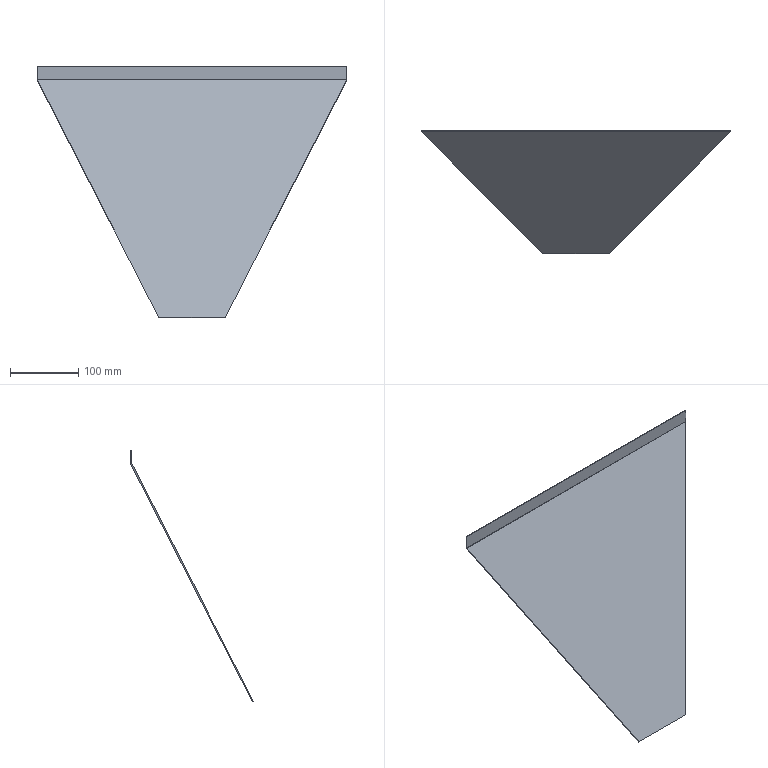Part | SolidWorks | features ICE 3, Blend 1, FlatPattern 1, SheetMetal 1, Shell 1, SolidToSheetMetal 1 | 1 solid | 14 faces | box 454 x 180.224 x 368.911 mm | volume 234028 mm3 | plane 10 | spline 2 | cylinder 2 | commonest cylinder face diameters 2 x1 6 x1
STEP:
#1=CARTESIAN_POINT('',(-226.89,228.671,-0.6434));
#2=VERTEX_POINT('',#1);
#3=CARTESIAN_POINT('',(-226.89,226.89,0.2673));
#4=VERTEX_POINT('',#3);
#5=CARTESIAN_POINT('',(-226.89,226.89,0.2673));
#6=DIRECTION('',(0.,-0.8903,0.4553));
#7=VECTOR('',#6,1000.);
#8=LINE('',#5,#7);
#9=EDGE_CURVE('',#2,#4,#8,.T.);
#10=ORIENTED_EDGE('',*,*,#9,.F.);
#11=CARTESIAN_POINT('',(-48.776,50.557,-348.911));
#12=VERTEX_POINT('',#11);
#13=CARTESIAN_POINT('',(-148.875,150.655,-153.188));
#14=DIRECTION('',(0.4144,-0.4144,-0.8103));
#15=VECTOR('',#14,1000.);
#16=LINE('',#13,#15);
#17=EDGE_CURVE('',#2,#12,#16,.T.);
#18=ORIENTED_EDGE('',*,*,#17,.T.);
#19=CARTESIAN_POINT('',(-48.776,48.776,-348.));
#20=VERTEX_POINT('',#19);
#21=CARTESIAN_POINT('',(-48.776,48.776,-348.));
#22=DIRECTION('',(0.,-0.8903,0.4553));
#23=VECTOR('',#22,1000.);
#24=LINE('',#21,#23);
#25=EDGE_CURVE('',#12,#20,#24,.T.);
#26=ORIENTED_EDGE('',*,*,#25,.T.);
#27=CARTESIAN_POINT('',(-148.875,148.875,-152.277));
#28=DIRECTION('',(0.4144,-0.4144,-0.8103));
#29=VECTOR('',#28,1000.);
#30=LINE('',#27,#29);
#31=EDGE_CURVE('',#4,#20,#30,.T.);
#32=ORIENTED_EDGE('',*,*,#31,.F.);
#33=EDGE_LOOP('',(#10,#18,#26,#32));
#34=FACE_OUTER_BOUND('',#33,.T.);
#35=CARTESIAN_POINT('',(-148.875,148.875,-152.277));
#36=DIRECTION('',(0.9101,0.1887,0.3689));
#37=DIRECTION('',(0.4144,-0.4144,-0.8103));
#38=AXIS2_PLACEMENT_3D('',#35,#36,#37);
#39=PLANE('',#38);
#40=ADVANCED_FACE('',(#34),#39,.F.);
#41=ORIENTED_EDGE('',*,*,#25,.F.);
#42=CARTESIAN_POINT('',(48.776,50.557,-348.911));
#43=VERTEX_POINT('',#42);
#44=CARTESIAN_POINT('',(0.,50.557,-348.911));
#45=DIRECTION('',(-1.,0.,0.));
#46=VECTOR('',#45,1000.);
#47=LINE('',#44,#46);
#48=EDGE_CURVE('',#43,#12,#47,.T.);
#49=ORIENTED_EDGE('',*,*,#48,.F.);
#50=CARTESIAN_POINT('',(48.776,48.776,-348.));
#51=VERTEX_POINT('',#50);
#52=CARTESIAN_POINT('',(48.776,48.776,-348.));
#53=DIRECTION('',(0.,-0.8903,0.4553));
#54=VECTOR('',#53,1000.);
#55=LINE('',#52,#54);
#56=EDGE_CURVE('',#43,#51,#55,.T.);
#57=ORIENTED_EDGE('',*,*,#56,.T.);
#58=CARTESIAN_POINT('',(0.,48.776,-348.));
#59=DIRECTION('',(-1.,0.,0.));
#60=VECTOR('',#59,1000.);
#61=LINE('',#58,#60);
#62=EDGE_CURVE('',#51,#20,#61,.T.);
#63=ORIENTED_EDGE('',*,*,#62,.T.);
#64=EDGE_LOOP('',(#41,#49,#57,#63));
#65=FACE_OUTER_BOUND('',#64,.T.);
#66=CARTESIAN_POINT('',(0.,48.776,-348.));
#67=DIRECTION('',(0.,-0.4553,-0.8903));
#68=DIRECTION('',(-1.,0.,0.));
#69=AXIS2_PLACEMENT_3D('',#66,#67,#68);
#70=PLANE('',#69);
#71=ADVANCED_FACE('',(#65),#70,.T.);
#72=ORIENTED_EDGE('',*,*,#56,.F.);
#73=CARTESIAN_POINT('',(226.89,228.671,-0.6434));
#74=VERTEX_POINT('',#73);
#75=CARTESIAN_POINT('',(148.875,150.655,-153.188));
#76=DIRECTION('',(-0.4144,-0.4144,-0.8103));
#77=VECTOR('',#76,1000.);
#78=LINE('',#75,#77);
#79=EDGE_CURVE('',#74,#43,#78,.T.);
#80=ORIENTED_EDGE('',*,*,#79,.F.);
#81=CARTESIAN_POINT('',(226.89,226.89,0.2673));
#82=VERTEX_POINT('',#81);
#83=CARTESIAN_POINT('',(226.89,226.89,0.2673));
#84=DIRECTION('',(0.,-0.8903,0.4553));
#85=VECTOR('',#84,1000.);
#86=LINE('',#83,#85);
#87=EDGE_CURVE('',#74,#82,#86,.T.);
#88=ORIENTED_EDGE('',*,*,#87,.T.);
#89=CARTESIAN_POINT('',(148.875,148.875,-152.277));
#90=DIRECTION('',(-0.4144,-0.4144,-0.8103));
#91=VECTOR('',#90,1000.);
#92=LINE('',#89,#91);
#93=EDGE_CURVE('',#82,#51,#92,.T.);
#94=ORIENTED_EDGE('',*,*,#93,.T.);
#95=EDGE_LOOP('',(#72,#80,#88,#94));
#96=FACE_OUTER_BOUND('',#95,.T.);
#97=CARTESIAN_POINT('',(148.875,148.875,-152.277));
#98=DIRECTION('',(0.9101,-0.1887,-0.3689));
#99=DIRECTION('',(-0.4144,-0.4144,-0.8103));
#100=AXIS2_PLACEMENT_3D('',#97,#98,#99);
#101=PLANE('',#100);
#102=ADVANCED_FACE('',(#96),#101,.T.);
#103=ORIENTED_EDGE('',*,*,#87,.F.);
#104=CARTESIAN_POINT('',(227.,229.,0.7226));
#105=VERTEX_POINT('',#104);
#106=CARTESIAN_POINT('',(226.89,228.671,-0.6434));
#107=CARTESIAN_POINT('',(226.963,228.888,-0.2185));
#108=CARTESIAN_POINT('',(227.,229.,0.2454));
#109=CARTESIAN_POINT('',(227.,229.,0.7226));
#110=(BOUNDED_CURVE()B_SPLINE_CURVE(3,(#106,#107,#108,#109),.UNSPECIFIED.,.F.,.F.)B_SPLINE_CURVE_WITH_KNOTS((4,4),(2.669,3.142),.UNSPECIFIED.)CURVE()GEOMETRIC_REPRESENTATION_ITEM()RATIONAL_B_SPLINE_CURVE((1.,0.9815,0.9815,1.))REPRESENTATION_ITEM(''));
#111=EDGE_CURVE('',#74,#105,#110,.T.);
#112=ORIENTED_EDGE('',*,*,#111,.T.);
#113=CARTESIAN_POINT('',(227.,227.,0.7226));
#114=VERTEX_POINT('',#113);
#115=CARTESIAN_POINT('',(227.,227.,0.7226));
#116=DIRECTION('',(0.,-1.,0.));
#117=VECTOR('',#116,1000.);
#118=LINE('',#115,#117);
#119=EDGE_CURVE('',#105,#114,#118,.T.);
#120=ORIENTED_EDGE('',*,*,#119,.T.);
#121=CARTESIAN_POINT('',(226.89,226.89,0.2673));
#122=CARTESIAN_POINT('',(226.963,226.963,0.4089));
#123=CARTESIAN_POINT('',(227.,227.,0.5636));
#124=CARTESIAN_POINT('',(227.,227.,0.7226));
#125=(BOUNDED_CURVE()B_SPLINE_CURVE(3,(#121,#122,#123,#124),.UNSPECIFIED.,.F.,.F.)B_SPLINE_CURVE_WITH_KNOTS((4,4),(2.669,3.142),.UNSPECIFIED.)CURVE()GEOMETRIC_REPRESENTATION_ITEM()RATIONAL_B_SPLINE_CURVE((1.,0.9815,0.9815,1.))REPRESENTATION_ITEM(''));
#126=EDGE_CURVE('',#82,#114,#125,.T.);
#127=ORIENTED_EDGE('',*,*,#126,.F.);
#128=EDGE_LOOP('',(#103,#112,#120,#127));
#129=FACE_OUTER_BOUND('',#128,.T.);
#130=CARTESIAN_POINT('',(225.,223.,0.7226));
#131=CARTESIAN_POINT('',(225.,223.667,0.7226));
#132=CARTESIAN_POINT('',(225.,224.333,0.7226));
#133=CARTESIAN_POINT('',(225.,225.,0.7226));
#134=CARTESIAN_POINT('',(225.,223.,-5.277));
#135=CARTESIAN_POINT('',(225.,223.667,-3.944));
#136=CARTESIAN_POINT('',(225.,224.333,-2.611));
#137=CARTESIAN_POINT('',(225.,225.,-1.277));
#138=CARTESIAN_POINT('',(227.,229.,-5.277));
#139=CARTESIAN_POINT('',(227.,228.333,-3.944));
#140=CARTESIAN_POINT('',(227.,227.667,-2.611));
#141=CARTESIAN_POINT('',(227.,227.,-1.277));
#142=CARTESIAN_POINT('',(227.,229.,0.7226));
#143=CARTESIAN_POINT('',(227.,228.333,0.7226));
#144=CARTESIAN_POINT('',(227.,227.667,0.7226));
#145=CARTESIAN_POINT('',(227.,227.,0.7226));
#146=CARTESIAN_POINT('',(227.,229.,6.723));
#147=CARTESIAN_POINT('',(227.,228.333,5.389));
#148=CARTESIAN_POINT('',(227.,227.667,4.056));
#149=CARTESIAN_POINT('',(227.,227.,2.723));
#150=CARTESIAN_POINT('',(225.,223.,6.723));
#151=CARTESIAN_POINT('',(225.,223.667,5.389));
#152=CARTESIAN_POINT('',(225.,224.333,4.056));
#153=CARTESIAN_POINT('',(225.,225.,2.723));
#154=CARTESIAN_POINT('',(225.,223.,0.7226));
#155=CARTESIAN_POINT('',(225.,223.667,0.7226));
#156=CARTESIAN_POINT('',(225.,224.333,0.7226));
#157=CARTESIAN_POINT('',(225.,225.,0.7226));
#158=(BOUNDED_SURFACE()B_SPLINE_SURFACE(3,3,((#130,#131,#132,#133),(#134,#135,#136,#137),(#138,#139,#140,#141),(#142,#143,#144,#145),(#146,#147,#148,#149),(#150,#151,#152,#153),(#154,#155,#156,#157)),.UNSPECIFIED.,.T.,.F.,.F.)B_SPLINE_SURFACE_WITH_KNOTS((4,3,4),(4,4),(0.,0.5,1.),(0.,1.),.UNSPECIFIED.)GEOMETRIC_REPRESENTATION_ITEM()RATIONAL_B_SPLINE_SURFACE(((1.,1.,1.,1.),(0.3333,0.3333,0.3333,0.3333),(0.3333,0.3333,0.3333,0.3333),(1.,1.,1.,1.),(0.3333,0.3333,0.3333,0.3333),(0.3333,0.3333,0.3333,0.3333),(1.,1.,1.,1.)))REPRESENTATION_ITEM('')SURFACE());
#159=ADVANCED_FACE('',(#129),#158,.T.);
#160=ORIENTED_EDGE('',*,*,#119,.F.);
#161=CARTESIAN_POINT('',(227.,229.,20.));
#162=VERTEX_POINT('',#161);
#163=CARTESIAN_POINT('',(227.,229.,20.));
#164=DIRECTION('',(0.,0.,-1.));
#165=VECTOR('',#164,1000.);
#166=LINE('',#163,#165);
#167=EDGE_CURVE('',#162,#105,#166,.T.);
#168=ORIENTED_EDGE('',*,*,#167,.F.);
#169=CARTESIAN_POINT('',(227.,227.,20.));
#170=VERTEX_POINT('',#169);
#171=CARTESIAN_POINT('',(227.,227.,20.));
#172=DIRECTION('',(0.,-1.,0.));
#173=VECTOR('',#172,1000.);
#174=LINE('',#171,#173);
#175=EDGE_CURVE('',#162,#170,#174,.T.);
#176=ORIENTED_EDGE('',*,*,#175,.T.);
#177=CARTESIAN_POINT('',(227.,227.,20.));
#178=DIRECTION('',(0.,0.,-1.));
#179=VECTOR('',#178,1000.);
#180=LINE('',#177,#179);
#181=EDGE_CURVE('',#170,#114,#180,.T.);
#182=ORIENTED_EDGE('',*,*,#181,.T.);
#183=EDGE_LOOP('',(#160,#168,#176,#182));
#184=FACE_OUTER_BOUND('',#183,.T.);
#185=CARTESIAN_POINT('',(227.,227.,20.));
#186=DIRECTION('',(-1.,0.,0.));
#187=DIRECTION('',(0.,0.,-1.));
#188=AXIS2_PLACEMENT_3D('',#185,#186,#187);
#189=PLANE('',#188);
#190=ADVANCED_FACE('',(#184),#189,.F.);
#191=ORIENTED_EDGE('',*,*,#175,.F.);
#192=CARTESIAN_POINT('',(-227.,229.,20.));
#193=VERTEX_POINT('',#192);
#194=CARTESIAN_POINT('',(229.,229.,20.));
#195=DIRECTION('',(-1.,0.,0.));
#196=VECTOR('',#195,1000.);
#197=LINE('',#194,#196);
#198=EDGE_CURVE('',#162,#193,#197,.T.);
#199=ORIENTED_EDGE('',*,*,#198,.T.);
#200=CARTESIAN_POINT('',(-227.,227.,20.));
#201=VERTEX_POINT('',#200);
#202=CARTESIAN_POINT('',(-227.,227.,20.));
#203=DIRECTION('',(0.,-1.,0.));
#204=VECTOR('',#203,1000.);
#205=LINE('',#202,#204);
#206=EDGE_CURVE('',#193,#201,#205,.T.);
#207=ORIENTED_EDGE('',*,*,#206,.T.);
#208=CARTESIAN_POINT('',(229.,227.,20.));
#209=DIRECTION('',(-1.,0.,0.));
#210=VECTOR('',#209,1000.);
#211=LINE('',#208,#210);
#212=EDGE_CURVE('',#170,#201,#211,.T.);
#213=ORIENTED_EDGE('',*,*,#212,.F.);
#214=EDGE_LOOP('',(#191,#199,#207,#213));
#215=FACE_OUTER_BOUND('',#214,.T.);
#216=CARTESIAN_POINT('',(229.,227.,20.));
#217=DIRECTION('',(0.,0.,1.));
#218=DIRECTION('',(-1.,0.,0.));
#219=AXIS2_PLACEMENT_3D('',#216,#217,#218);
#220=PLANE('',#219);
#221=ADVANCED_FACE('',(#215),#220,.T.);
#222=ORIENTED_EDGE('',*,*,#206,.F.);
#223=CARTESIAN_POINT('',(-227.,229.,0.7226));
#224=VERTEX_POINT('',#223);
#225=CARTESIAN_POINT('',(-227.,229.,20.));
#226=DIRECTION('',(0.,0.,-1.));
#227=VECTOR('',#226,1000.);
#228=LINE('',#225,#227);
#229=EDGE_CURVE('',#193,#224,#228,.T.);
#230=ORIENTED_EDGE('',*,*,#229,.T.);
#231=CARTESIAN_POINT('',(-227.,227.,0.7226));
#232=VERTEX_POINT('',#231);
#233=CARTESIAN_POINT('',(-227.,227.,0.7226));
#234=DIRECTION('',(0.,-1.,0.));
#235=VECTOR('',#234,1000.);
#236=LINE('',#233,#235);
#237=EDGE_CURVE('',#224,#232,#236,.T.);
#238=ORIENTED_EDGE('',*,*,#237,.T.);
#239=CARTESIAN_POINT('',(-227.,227.,20.));
#240=DIRECTION('',(0.,0.,-1.));
#241=VECTOR('',#240,1000.);
#242=LINE('',#239,#241);
#243=EDGE_CURVE('',#201,#232,#242,.T.);
#244=ORIENTED_EDGE('',*,*,#243,.F.);
#245=EDGE_LOOP('',(#222,#230,#238,#244));
#246=FACE_OUTER_BOUND('',#245,.T.);
#247=CARTESIAN_POINT('',(-227.,227.,20.));
#248=DIRECTION('',(-1.,0.,0.));
#249=DIRECTION('',(0.,0.,-1.));
#250=AXIS2_PLACEMENT_3D('',#247,#248,#249);
#251=PLANE('',#250);
#252=ADVANCED_FACE('',(#246),#251,.T.);
#253=CARTESIAN_POINT('',(-227.,229.,0.7226));
#254=CARTESIAN_POINT('',(-227.,229.,0.2454));
#255=CARTESIAN_POINT('',(-226.963,228.888,-0.2185));
#256=CARTESIAN_POINT('',(-226.89,228.671,-0.6434));
#257=(BOUNDED_CURVE()B_SPLINE_CURVE(3,(#253,#254,#255,#256),.UNSPECIFIED.,.F.,.F.)B_SPLINE_CURVE_WITH_KNOTS((4,4),(0.,0.4727),.UNSPECIFIED.)CURVE()GEOMETRIC_REPRESENTATION_ITEM()RATIONAL_B_SPLINE_CURVE((1.,0.9815,0.9815,1.))REPRESENTATION_ITEM(''));
#258=EDGE_CURVE('',#224,#2,#257,.T.);
#259=ORIENTED_EDGE('',*,*,#258,.T.);
#260=ORIENTED_EDGE('',*,*,#9,.T.);
#261=CARTESIAN_POINT('',(-227.,227.,0.7226));
#262=CARTESIAN_POINT('',(-227.,227.,0.5636));
#263=CARTESIAN_POINT('',(-226.963,226.963,0.4089));
#264=CARTESIAN_POINT('',(-226.89,226.89,0.2673));
#265=(BOUNDED_CURVE()B_SPLINE_CURVE(3,(#261,#262,#263,#264),.UNSPECIFIED.,.F.,.F.)B_SPLINE_CURVE_WITH_KNOTS((4,4),(0.,0.4727),.UNSPECIFIED.)CURVE()GEOMETRIC_REPRESENTATION_ITEM()RATIONAL_B_SPLINE_CURVE((1.,0.9815,0.9815,1.))REPRESENTATION_ITEM(''));
#266=EDGE_CURVE('',#232,#4,#265,.T.);
#267=ORIENTED_EDGE('',*,*,#266,.F.);
#268=ORIENTED_EDGE('',*,*,#237,.F.);
#269=EDGE_LOOP('',(#259,#260,#267,#268));
#270=FACE_OUTER_BOUND('',#269,.T.);
#271=CARTESIAN_POINT('',(-227.,229.,0.7226));
#272=CARTESIAN_POINT('',(-227.,228.333,0.7226));
#273=CARTESIAN_POINT('',(-227.,227.667,0.7226));
#274=CARTESIAN_POINT('',(-227.,227.,0.7226));
#275=CARTESIAN_POINT('',(-227.,229.,-5.277));
#276=CARTESIAN_POINT('',(-227.,228.333,-3.944));
#277=CARTESIAN_POINT('',(-227.,227.667,-2.611));
#278=CARTESIAN_POINT('',(-227.,227.,-1.277));
#279=CARTESIAN_POINT('',(-225.,223.,-5.277));
#280=CARTESIAN_POINT('',(-225.,223.667,-3.944));
#281=CARTESIAN_POINT('',(-225.,224.333,-2.611));
#282=CARTESIAN_POINT('',(-225.,225.,-1.277));
#283=CARTESIAN_POINT('',(-225.,223.,0.7226));
#284=CARTESIAN_POINT('',(-225.,223.667,0.7226));
#285=CARTESIAN_POINT('',(-225.,224.333,0.7226));
#286=CARTESIAN_POINT('',(-225.,225.,0.7226));
#287=CARTESIAN_POINT('',(-225.,223.,6.723));
#288=CARTESIAN_POINT('',(-225.,223.667,5.389));
#289=CARTESIAN_POINT('',(-225.,224.333,4.056));
#290=CARTESIAN_POINT('',(-225.,225.,2.723));
#291=CARTESIAN_POINT('',(-227.,229.,6.723));
#292=CARTESIAN_POINT('',(-227.,228.333,5.389));
#293=CARTESIAN_POINT('',(-227.,227.667,4.056));
#294=CARTESIAN_POINT('',(-227.,227.,2.723));
#295=CARTESIAN_POINT('',(-227.,229.,0.7226));
#296=CARTESIAN_POINT('',(-227.,228.333,0.7226));
#297=CARTESIAN_POINT('',(-227.,227.667,0.7226));
#298=CARTESIAN_POINT('',(-227.,227.,0.7226));
#299=(BOUNDED_SURFACE()B_SPLINE_SURFACE(3,3,((#271,#272,#273,#274),(#275,#276,#277,#278),(#279,#280,#281,#282),(#283,#284,#285,#286),(#287,#288,#289,#290),(#291,#292,#293,#294),(#295,#296,#297,#298)),.UNSPECIFIED.,.T.,.F.,.F.)B_SPLINE_SURFACE_WITH_KNOTS((4,3,4),(4,4),(0.,0.5,1.),(0.,1.),.UNSPECIFIED.)GEOMETRIC_REPRESENTATION_ITEM()RATIONAL_B_SPLINE_SURFACE(((1.,1.,1.,1.),(0.3333,0.3333,0.3333,0.3333),(0.3333,0.3333,0.3333,0.3333),(1.,1.,1.,1.),(0.3333,0.3333,0.3333,0.3333),(0.3333,0.3333,0.3333,0.3333),(1.,1.,1.,1.)))REPRESENTATION_ITEM('')SURFACE());
#300=ADVANCED_FACE('',(#270),#299,.T.);
#301=ORIENTED_EDGE('',*,*,#243,.T.);
#302=CARTESIAN_POINT('',(229.,227.,0.7226));
#303=DIRECTION('',(1.,0.,0.));
#304=VECTOR('',#303,1000.);
#305=LINE('',#302,#304);
#306=EDGE_CURVE('',#232,#114,#305,.T.);
#307=ORIENTED_EDGE('',*,*,#306,.T.);
#308=ORIENTED_EDGE('',*,*,#181,.F.);
#309=ORIENTED_EDGE('',*,*,#212,.T.);
#310=EDGE_LOOP('',(#301,#307,#308,#309));
#311=FACE_OUTER_BOUND('',#310,.T.);
#312=CARTESIAN_POINT('',(229.,227.,20.));
#313=DIRECTION('',(0.,-1.,0.));
#314=DIRECTION('',(0.,0.,-1.));
#315=AXIS2_PLACEMENT_3D('',#312,#313,#314);
#316=PLANE('',#315);
#317=ADVANCED_FACE('',(#311),#316,.T.);
#318=ORIENTED_EDGE('',*,*,#93,.F.);
#319=CARTESIAN_POINT('',(0.,226.89,0.2673));
#320=DIRECTION('',(-1.,0.,0.));
#321=VECTOR('',#320,1000.);
#322=LINE('',#319,#321);
#323=EDGE_CURVE('',#82,#4,#322,.T.);
#324=ORIENTED_EDGE('',*,*,#323,.T.);
#325=ORIENTED_EDGE('',*,*,#31,.T.);
#326=ORIENTED_EDGE('',*,*,#62,.F.);
#327=EDGE_LOOP('',(#318,#324,#325,#326));
#328=FACE_OUTER_BOUND('',#327,.T.);
#329=CARTESIAN_POINT('',(0.,179.741,-91.925));
#330=DIRECTION('',(0.,0.8903,-0.4553));
#331=DIRECTION('',(0.,0.4553,0.8903));
#332=AXIS2_PLACEMENT_3D('',#329,#330,#331);
#333=PLANE('',#332);
#334=ADVANCED_FACE('',(#328),#333,.F.);
#335=ORIENTED_EDGE('',*,*,#126,.T.);
#336=ORIENTED_EDGE('',*,*,#306,.F.);
#337=ORIENTED_EDGE('',*,*,#266,.T.);
#338=ORIENTED_EDGE('',*,*,#323,.F.);
#339=EDGE_LOOP('',(#335,#336,#337,#338));
#340=FACE_OUTER_BOUND('',#339,.T.);
#341=CARTESIAN_POINT('',(0.,226.,0.7226));
#342=DIRECTION('',(-1.,0.,0.));
#343=DIRECTION('',(0.,0.,1.));
#344=AXIS2_PLACEMENT_3D('',#341,#342,#343);
#345=CYLINDRICAL_SURFACE('',#344,1.);
#346=ADVANCED_FACE('',(#340),#345,.F.);
#347=ORIENTED_EDGE('',*,*,#229,.F.);
#348=ORIENTED_EDGE('',*,*,#198,.F.);
#349=ORIENTED_EDGE('',*,*,#167,.T.);
#350=CARTESIAN_POINT('',(229.,229.,0.7226));
#351=DIRECTION('',(1.,0.,0.));
#352=VECTOR('',#351,1000.);
#353=LINE('',#350,#352);
#354=EDGE_CURVE('',#224,#105,#353,.T.);
#355=ORIENTED_EDGE('',*,*,#354,.F.);
#356=EDGE_LOOP('',(#347,#348,#349,#355));
#357=FACE_OUTER_BOUND('',#356,.T.);
#358=CARTESIAN_POINT('',(229.,229.,20.));
#359=DIRECTION('',(0.,-1.,0.));
#360=DIRECTION('',(0.,0.,-1.));
#361=AXIS2_PLACEMENT_3D('',#358,#359,#360);
#362=PLANE('',#361);
#363=ADVANCED_FACE('',(#357),#362,.F.);
#364=ORIENTED_EDGE('',*,*,#79,.T.);
#365=ORIENTED_EDGE('',*,*,#48,.T.);
#366=ORIENTED_EDGE('',*,*,#17,.F.);
#367=CARTESIAN_POINT('',(0.,228.671,-0.6434));
#368=DIRECTION('',(-1.,0.,0.));
#369=VECTOR('',#368,1000.);
#370=LINE('',#367,#369);
#371=EDGE_CURVE('',#74,#2,#370,.T.);
#372=ORIENTED_EDGE('',*,*,#371,.F.);
#373=EDGE_LOOP('',(#364,#365,#366,#372));
#374=FACE_OUTER_BOUND('',#373,.T.);
#375=CARTESIAN_POINT('',(0.,181.521,-92.835));
#376=DIRECTION('',(0.,0.8903,-0.4553));
#377=DIRECTION('',(0.,0.4553,0.8903));
#378=AXIS2_PLACEMENT_3D('',#375,#376,#377);
#379=PLANE('',#378);
#380=ADVANCED_FACE('',(#374),#379,.T.);
#381=ORIENTED_EDGE('',*,*,#111,.F.);
#382=ORIENTED_EDGE('',*,*,#371,.T.);
#383=ORIENTED_EDGE('',*,*,#258,.F.);
#384=ORIENTED_EDGE('',*,*,#354,.T.);
#385=EDGE_LOOP('',(#381,#382,#383,#384));
#386=FACE_OUTER_BOUND('',#385,.T.);
#387=CARTESIAN_POINT('',(0.,226.,0.7226));
#388=DIRECTION('',(-1.,0.,0.));
#389=DIRECTION('',(0.,0.,1.));
#390=AXIS2_PLACEMENT_3D('',#387,#388,#389);
#391=CYLINDRICAL_SURFACE('',#390,3.);
#392=ADVANCED_FACE('',(#386),#391,.T.);
#393=CLOSED_SHELL('',(#40,#71,#102,#159,#190,#221,#252,#300,#317,#334,#346,#363,#380,#392));
#394=MANIFOLD_SOLID_BREP('',#393);
#395=CARTESIAN_POINT('',(0.,0.,0.));
#396=DIRECTION('',(0.,0.,1.));
#397=DIRECTION('',(1.,0.,0.));
#398=AXIS2_PLACEMENT_3D('',#395,#396,#397);
#399=(LENGTH_UNIT()NAMED_UNIT(*)SI_UNIT(.MILLI.,.METRE.));
#400=UNCERTAINTY_MEASURE_WITH_UNIT(LENGTH_MEASURE(0.00001),#399,'','');
#401=(NAMED_UNIT(*)PLANE_ANGLE_UNIT()SI_UNIT($,.RADIAN.));
#402=(NAMED_UNIT(*)SI_UNIT($,.STERADIAN.)SOLID_ANGLE_UNIT());
#403=(GEOMETRIC_REPRESENTATION_CONTEXT(3)GLOBAL_UNCERTAINTY_ASSIGNED_CONTEXT((#400))GLOBAL_UNIT_ASSIGNED_CONTEXT((#399,#401,#402))REPRESENTATION_CONTEXT('',''));
#404=ADVANCED_BREP_SHAPE_REPRESENTATION('',(#394,#398),#403);